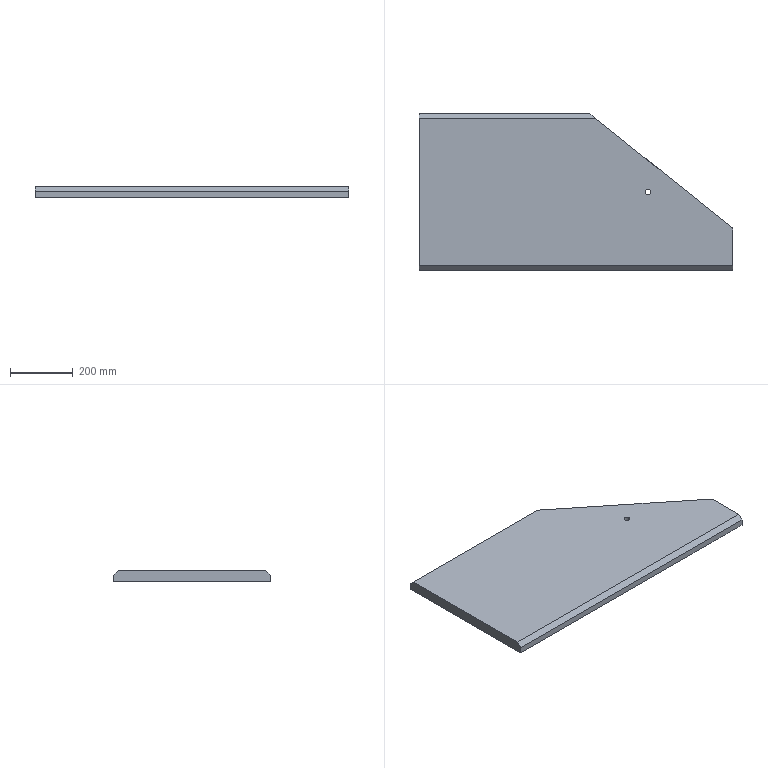Part | SolidWorks | features 3DProfileFeature 1, Chamfer 1, Cut 1, Extrusion 1, HoleWzd 1 | 1 solid | 11 faces | box 1000 x 500 x 35 mm | volume 14402910 mm3 | plane 9 | cylinder 2 | commonest cylinder face diameters 17.5 x2
STEP:
#1=CARTESIAN_POINT('',(-278.75,-275.,-35.));
#2=VERTEX_POINT('',#1);
#3=CARTESIAN_POINT('',(-261.25,-275.,-35.));
#4=VERTEX_POINT('',#3);
#5=CARTESIAN_POINT('',(-270.,-275.,-35.));
#6=DIRECTION('',(0.,0.,1.));
#7=DIRECTION('',(1.,0.,0.));
#8=AXIS2_PLACEMENT_3D('',#5,#6,#7);
#9=CIRCLE('',#8,8.75);
#10=EDGE_CURVE('',#2,#4,#9,.T.);
#11=ORIENTED_EDGE('',*,*,#10,.F.);
#12=CARTESIAN_POINT('',(-278.75,-275.,0.));
#13=VERTEX_POINT('',#12);
#14=CARTESIAN_POINT('',(-278.75,-275.,0.));
#15=DIRECTION('',(0.,0.,1.));
#16=VECTOR('',#15,1000.);
#17=LINE('',#14,#16);
#18=EDGE_CURVE('',#2,#13,#17,.T.);
#19=ORIENTED_EDGE('',*,*,#18,.T.);
#20=CARTESIAN_POINT('',(-261.25,-275.,0.));
#21=VERTEX_POINT('',#20);
#22=CARTESIAN_POINT('',(-270.,-275.,0.));
#23=DIRECTION('',(0.,0.,1.));
#24=DIRECTION('',(1.,0.,0.));
#25=AXIS2_PLACEMENT_3D('',#22,#23,#24);
#26=CIRCLE('',#25,8.75);
#27=EDGE_CURVE('',#13,#21,#26,.T.);
#28=ORIENTED_EDGE('',*,*,#27,.T.);
#29=CARTESIAN_POINT('',(-261.25,-275.,0.));
#30=DIRECTION('',(0.,0.,1.));
#31=VECTOR('',#30,1000.);
#32=LINE('',#29,#31);
#33=EDGE_CURVE('',#4,#21,#32,.T.);
#34=ORIENTED_EDGE('',*,*,#33,.F.);
#35=EDGE_LOOP('',(#11,#19,#28,#34));
#36=FACE_OUTER_BOUND('',#35,.T.);
#37=CARTESIAN_POINT('',(-270.,-275.,0.));
#38=DIRECTION('',(0.,0.,1.));
#39=DIRECTION('',(1.,0.,0.));
#40=AXIS2_PLACEMENT_3D('',#37,#38,#39);
#41=CYLINDRICAL_SURFACE('',#40,8.75);
#42=ADVANCED_FACE('',(#36),#41,.F.);
#43=CARTESIAN_POINT('',(0.,-390.,-35.));
#44=VERTEX_POINT('',#43);
#45=CARTESIAN_POINT('',(0.,-390.,0.));
#46=VERTEX_POINT('',#45);
#47=CARTESIAN_POINT('',(0.,-390.,-35.));
#48=DIRECTION('',(0.,0.,1.));
#49=VECTOR('',#48,1000.);
#50=LINE('',#47,#49);
#51=EDGE_CURVE('',#44,#46,#50,.T.);
#52=ORIENTED_EDGE('',*,*,#51,.T.);
#53=CARTESIAN_POINT('',(0.,-510.,0.));
#54=VERTEX_POINT('',#53);
#55=CARTESIAN_POINT('',(0.,-25.,0.));
#56=DIRECTION('',(0.,1.,0.));
#57=VECTOR('',#56,1000.);
#58=LINE('',#55,#57);
#59=EDGE_CURVE('',#54,#46,#58,.T.);
#60=ORIENTED_EDGE('',*,*,#59,.F.);
#61=CARTESIAN_POINT('',(0.,-525.,-15.));
#62=VERTEX_POINT('',#61);
#63=CARTESIAN_POINT('',(0.,-285.,225.));
#64=DIRECTION('',(0.,-0.7071,-0.7071));
#65=VECTOR('',#64,1000.);
#66=LINE('',#63,#65);
#67=EDGE_CURVE('',#54,#62,#66,.T.);
#68=ORIENTED_EDGE('',*,*,#67,.T.);
#69=CARTESIAN_POINT('',(0.,-525.,-35.));
#70=VERTEX_POINT('',#69);
#71=CARTESIAN_POINT('',(0.,-525.,-35.));
#72=DIRECTION('',(0.,0.,1.));
#73=VECTOR('',#72,1000.);
#74=LINE('',#71,#73);
#75=EDGE_CURVE('',#70,#62,#74,.T.);
#76=ORIENTED_EDGE('',*,*,#75,.F.);
#77=CARTESIAN_POINT('',(0.,-25.,-35.));
#78=DIRECTION('',(0.,1.,0.));
#79=VECTOR('',#78,1000.);
#80=LINE('',#77,#79);
#81=EDGE_CURVE('',#70,#44,#80,.T.);
#82=ORIENTED_EDGE('',*,*,#81,.T.);
#83=EDGE_LOOP('',(#52,#60,#68,#76,#82));
#84=FACE_OUTER_BOUND('',#83,.T.);
#85=CARTESIAN_POINT('',(0.,-25.,-35.));
#86=DIRECTION('',(1.,0.,0.));
#87=DIRECTION('',(0.,1.,0.));
#88=AXIS2_PLACEMENT_3D('',#85,#86,#87);
#89=PLANE('',#88);
#90=ADVANCED_FACE('',(#84),#89,.T.);
#91=ORIENTED_EDGE('',*,*,#75,.T.);
#92=CARTESIAN_POINT('',(-1000.,-525.,-15.));
#93=VERTEX_POINT('',#92);
#94=CARTESIAN_POINT('',(-1000.,-525.,-15.));
#95=DIRECTION('',(-1.,0.,0.));
#96=VECTOR('',#95,1000.);
#97=LINE('',#94,#96);
#98=EDGE_CURVE('',#62,#93,#97,.T.);
#99=ORIENTED_EDGE('',*,*,#98,.T.);
#100=CARTESIAN_POINT('',(-1000.,-525.,-35.));
#101=VERTEX_POINT('',#100);
#102=CARTESIAN_POINT('',(-1000.,-525.,-35.));
#103=DIRECTION('',(0.,0.,1.));
#104=VECTOR('',#103,1000.);
#105=LINE('',#102,#104);
#106=EDGE_CURVE('',#101,#93,#105,.T.);
#107=ORIENTED_EDGE('',*,*,#106,.F.);
#108=CARTESIAN_POINT('',(0.,-525.,-35.));
#109=DIRECTION('',(1.,0.,0.));
#110=VECTOR('',#109,1000.);
#111=LINE('',#108,#110);
#112=EDGE_CURVE('',#101,#70,#111,.T.);
#113=ORIENTED_EDGE('',*,*,#112,.T.);
#114=EDGE_LOOP('',(#91,#99,#107,#113));
#115=FACE_OUTER_BOUND('',#114,.T.);
#116=CARTESIAN_POINT('',(0.,-525.,-35.));
#117=DIRECTION('',(0.,-1.,0.));
#118=DIRECTION('',(1.,0.,0.));
#119=AXIS2_PLACEMENT_3D('',#116,#117,#118);
#120=PLANE('',#119);
#121=ADVANCED_FACE('',(#115),#120,.T.);
#122=CARTESIAN_POINT('',(-1000.,-40.,0.));
#123=VERTEX_POINT('',#122);
#124=CARTESIAN_POINT('',(-1000.,-510.,0.));
#125=VERTEX_POINT('',#124);
#126=CARTESIAN_POINT('',(-1000.,-25.,0.));
#127=DIRECTION('',(0.,-1.,0.));
#128=VECTOR('',#127,1000.);
#129=LINE('',#126,#128);
#130=EDGE_CURVE('',#123,#125,#129,.T.);
#131=ORIENTED_EDGE('',*,*,#130,.F.);
#132=CARTESIAN_POINT('',(-1000.,-25.,-15.));
#133=VERTEX_POINT('',#132);
#134=CARTESIAN_POINT('',(-1000.,-15.,-25.));
#135=DIRECTION('',(0.,0.7071,-0.7071));
#136=VECTOR('',#135,1000.);
#137=LINE('',#134,#136);
#138=EDGE_CURVE('',#123,#133,#137,.T.);
#139=ORIENTED_EDGE('',*,*,#138,.T.);
#140=CARTESIAN_POINT('',(-1000.,-25.,-35.));
#141=VERTEX_POINT('',#140);
#142=CARTESIAN_POINT('',(-1000.,-25.,-35.));
#143=DIRECTION('',(0.,0.,1.));
#144=VECTOR('',#143,1000.);
#145=LINE('',#142,#144);
#146=EDGE_CURVE('',#141,#133,#145,.T.);
#147=ORIENTED_EDGE('',*,*,#146,.F.);
#148=CARTESIAN_POINT('',(-1000.,-25.,-35.));
#149=DIRECTION('',(0.,-1.,0.));
#150=VECTOR('',#149,1000.);
#151=LINE('',#148,#150);
#152=EDGE_CURVE('',#141,#101,#151,.T.);
#153=ORIENTED_EDGE('',*,*,#152,.T.);
#154=ORIENTED_EDGE('',*,*,#106,.T.);
#155=CARTESIAN_POINT('',(-1000.,-285.,225.));
#156=DIRECTION('',(0.,0.7071,0.7071));
#157=VECTOR('',#156,1000.);
#158=LINE('',#155,#157);
#159=EDGE_CURVE('',#93,#125,#158,.T.);
#160=ORIENTED_EDGE('',*,*,#159,.T.);
#161=EDGE_LOOP('',(#131,#139,#147,#153,#154,#160));
#162=FACE_OUTER_BOUND('',#161,.T.);
#163=CARTESIAN_POINT('',(-1000.,-25.,-35.));
#164=DIRECTION('',(-1.,0.,0.));
#165=DIRECTION('',(0.,-1.,0.));
#166=AXIS2_PLACEMENT_3D('',#163,#164,#165);
#167=PLANE('',#166);
#168=ADVANCED_FACE('',(#162),#167,.T.);
#169=CARTESIAN_POINT('',(-456.25,-25.,-35.));
#170=VERTEX_POINT('',#169);
#171=CARTESIAN_POINT('',(-456.25,-25.,-15.));
#172=VERTEX_POINT('',#171);
#173=CARTESIAN_POINT('',(-456.25,-25.,-35.));
#174=DIRECTION('',(0.,0.,1.));
#175=VECTOR('',#174,1000.);
#176=LINE('',#173,#175);
#177=EDGE_CURVE('',#170,#172,#176,.T.);
#178=ORIENTED_EDGE('',*,*,#177,.F.);
#179=CARTESIAN_POINT('',(0.,-25.,-35.));
#180=DIRECTION('',(-1.,0.,0.));
#181=VECTOR('',#180,1000.);
#182=LINE('',#179,#181);
#183=EDGE_CURVE('',#170,#141,#182,.T.);
#184=ORIENTED_EDGE('',*,*,#183,.T.);
#185=ORIENTED_EDGE('',*,*,#146,.T.);
#186=CARTESIAN_POINT('',(0.,-25.,-15.));
#187=DIRECTION('',(1.,0.,0.));
#188=VECTOR('',#187,1000.);
#189=LINE('',#186,#188);
#190=EDGE_CURVE('',#133,#172,#189,.T.);
#191=ORIENTED_EDGE('',*,*,#190,.T.);
#192=EDGE_LOOP('',(#178,#184,#185,#191));
#193=FACE_OUTER_BOUND('',#192,.T.);
#194=CARTESIAN_POINT('',(0.,-25.,-35.));
#195=DIRECTION('',(0.,1.,0.));
#196=DIRECTION('',(-1.,0.,0.));
#197=AXIS2_PLACEMENT_3D('',#194,#195,#196);
#198=PLANE('',#197);
#199=ADVANCED_FACE('',(#193),#198,.T.);
#200=CARTESIAN_POINT('',(0.,-390.,-35.));
#201=DIRECTION('',(0.7809,-0.6247,0.));
#202=VECTOR('',#201,1000.);
#203=LINE('',#200,#202);
#204=EDGE_CURVE('',#170,#44,#203,.T.);
#205=ORIENTED_EDGE('',*,*,#204,.T.);
#206=ORIENTED_EDGE('',*,*,#81,.F.);
#207=ORIENTED_EDGE('',*,*,#112,.F.);
#208=ORIENTED_EDGE('',*,*,#152,.F.);
#209=ORIENTED_EDGE('',*,*,#183,.F.);
#210=EDGE_LOOP('',(#205,#206,#207,#208,#209));
#211=FACE_OUTER_BOUND('',#210,.T.);
#212=CARTESIAN_POINT('',(-270.,-275.,-35.));
#213=DIRECTION('',(0.,0.,1.));
#214=DIRECTION('',(1.,0.,0.));
#215=AXIS2_PLACEMENT_3D('',#212,#213,#214);
#216=CIRCLE('',#215,8.75);
#217=EDGE_CURVE('',#4,#2,#216,.T.);
#218=ORIENTED_EDGE('',*,*,#217,.T.);
#219=ORIENTED_EDGE('',*,*,#10,.T.);
#220=EDGE_LOOP('',(#218,#219));
#221=FACE_BOUND('',#220,.T.);
#222=CARTESIAN_POINT('',(0.,0.,-35.));
#223=DIRECTION('',(0.,0.,-1.));
#224=DIRECTION('',(-1.,0.,0.));
#225=AXIS2_PLACEMENT_3D('',#222,#223,#224);
#226=PLANE('',#225);
#227=ADVANCED_FACE('',(#211,#221),#226,.T.);
#228=CARTESIAN_POINT('',(-270.,-275.,0.));
#229=DIRECTION('',(0.,0.,1.));
#230=DIRECTION('',(1.,0.,0.));
#231=AXIS2_PLACEMENT_3D('',#228,#229,#230);
#232=CIRCLE('',#231,8.75);
#233=EDGE_CURVE('',#21,#13,#232,.T.);
#234=ORIENTED_EDGE('',*,*,#233,.F.);
#235=ORIENTED_EDGE('',*,*,#27,.F.);
#236=EDGE_LOOP('',(#234,#235));
#237=FACE_BOUND('',#236,.T.);
#238=ORIENTED_EDGE('',*,*,#59,.T.);
#239=CARTESIAN_POINT('',(-437.5,-40.,0.));
#240=VERTEX_POINT('',#239);
#241=CARTESIAN_POINT('',(0.,-390.,0.));
#242=DIRECTION('',(0.7809,-0.6247,0.));
#243=VECTOR('',#242,1000.);
#244=LINE('',#241,#243);
#245=EDGE_CURVE('',#240,#46,#244,.T.);
#246=ORIENTED_EDGE('',*,*,#245,.F.);
#247=CARTESIAN_POINT('',(-1000.,-40.,0.));
#248=DIRECTION('',(-1.,0.,0.));
#249=VECTOR('',#248,1000.);
#250=LINE('',#247,#249);
#251=EDGE_CURVE('',#240,#123,#250,.T.);
#252=ORIENTED_EDGE('',*,*,#251,.T.);
#253=ORIENTED_EDGE('',*,*,#130,.T.);
#254=CARTESIAN_POINT('',(0.,-510.,0.));
#255=DIRECTION('',(1.,0.,0.));
#256=VECTOR('',#255,1000.);
#257=LINE('',#254,#256);
#258=EDGE_CURVE('',#125,#54,#257,.T.);
#259=ORIENTED_EDGE('',*,*,#258,.T.);
#260=EDGE_LOOP('',(#238,#246,#252,#253,#259));
#261=FACE_OUTER_BOUND('',#260,.T.);
#262=CARTESIAN_POINT('',(0.,0.,0.));
#263=DIRECTION('',(0.,0.,-1.));
#264=DIRECTION('',(-1.,0.,0.));
#265=AXIS2_PLACEMENT_3D('',#262,#263,#264);
#266=PLANE('',#265);
#267=ADVANCED_FACE('',(#237,#261),#266,.F.);
#268=ORIENTED_EDGE('',*,*,#18,.F.);
#269=ORIENTED_EDGE('',*,*,#217,.F.);
#270=ORIENTED_EDGE('',*,*,#33,.T.);
#271=ORIENTED_EDGE('',*,*,#233,.T.);
#272=EDGE_LOOP('',(#268,#269,#270,#271));
#273=FACE_OUTER_BOUND('',#272,.T.);
#274=CARTESIAN_POINT('',(-270.,-275.,0.));
#275=DIRECTION('',(0.,0.,1.));
#276=DIRECTION('',(1.,0.,0.));
#277=AXIS2_PLACEMENT_3D('',#274,#275,#276);
#278=CYLINDRICAL_SURFACE('',#277,8.75);
#279=ADVANCED_FACE('',(#273),#278,.F.);
#280=CARTESIAN_POINT('',(-245.614,-193.509,153.509));
#281=DIRECTION('',(0.6623,-0.5298,0.5298));
#282=VECTOR('',#281,1000.);
#283=LINE('',#280,#282);
#284=EDGE_CURVE('',#172,#240,#283,.T.);
#285=ORIENTED_EDGE('',*,*,#284,.F.);
#286=ORIENTED_EDGE('',*,*,#190,.F.);
#287=ORIENTED_EDGE('',*,*,#138,.F.);
#288=ORIENTED_EDGE('',*,*,#251,.F.);
#289=EDGE_LOOP('',(#285,#286,#287,#288));
#290=FACE_OUTER_BOUND('',#289,.T.);
#291=CARTESIAN_POINT('',(0.,-40.,0.));
#292=DIRECTION('',(0.,0.7071,0.7071));
#293=DIRECTION('',(1.,0.,0.));
#294=AXIS2_PLACEMENT_3D('',#291,#292,#293);
#295=PLANE('',#294);
#296=ADVANCED_FACE('',(#290),#295,.T.);
#297=ORIENTED_EDGE('',*,*,#159,.F.);
#298=ORIENTED_EDGE('',*,*,#98,.F.);
#299=ORIENTED_EDGE('',*,*,#67,.F.);
#300=ORIENTED_EDGE('',*,*,#258,.F.);
#301=EDGE_LOOP('',(#297,#298,#299,#300));
#302=FACE_OUTER_BOUND('',#301,.T.);
#303=CARTESIAN_POINT('',(0.,-510.,0.));
#304=DIRECTION('',(0.,-0.7071,0.7071));
#305=DIRECTION('',(-1.,0.,0.));
#306=AXIS2_PLACEMENT_3D('',#303,#304,#305);
#307=PLANE('',#306);
#308=ADVANCED_FACE('',(#302),#307,.T.);
#309=ORIENTED_EDGE('',*,*,#177,.T.);
#310=ORIENTED_EDGE('',*,*,#284,.T.);
#311=ORIENTED_EDGE('',*,*,#245,.T.);
#312=ORIENTED_EDGE('',*,*,#51,.F.);
#313=ORIENTED_EDGE('',*,*,#204,.F.);
#314=EDGE_LOOP('',(#309,#310,#311,#312,#313));
#315=FACE_OUTER_BOUND('',#314,.T.);
#316=CARTESIAN_POINT('',(0.,-390.,-35.));
#317=DIRECTION('',(-0.6247,-0.7809,0.));
#318=DIRECTION('',(0.7809,-0.6247,0.));
#319=AXIS2_PLACEMENT_3D('',#316,#317,#318);
#320=PLANE('',#319);
#321=ADVANCED_FACE('',(#315),#320,.F.);
#322=CLOSED_SHELL('',(#42,#90,#121,#168,#199,#227,#267,#279,#296,#308,#321));
#323=MANIFOLD_SOLID_BREP('',#322);
#324=CARTESIAN_POINT('',(0.,0.,0.));
#325=DIRECTION('',(0.,0.,1.));
#326=DIRECTION('',(1.,0.,0.));
#327=AXIS2_PLACEMENT_3D('',#324,#325,#326);
#328=(LENGTH_UNIT()NAMED_UNIT(*)SI_UNIT(.MILLI.,.METRE.));
#329=UNCERTAINTY_MEASURE_WITH_UNIT(LENGTH_MEASURE(0.00001),#328,'','');
#330=(NAMED_UNIT(*)PLANE_ANGLE_UNIT()SI_UNIT($,.RADIAN.));
#331=(NAMED_UNIT(*)SI_UNIT($,.STERADIAN.)SOLID_ANGLE_UNIT());
#332=(GEOMETRIC_REPRESENTATION_CONTEXT(3)GLOBAL_UNCERTAINTY_ASSIGNED_CONTEXT((#329))GLOBAL_UNIT_ASSIGNED_CONTEXT((#328,#330,#331))REPRESENTATION_CONTEXT('',''));
#333=ADVANCED_BREP_SHAPE_REPRESENTATION('',(#323,#327),#332);